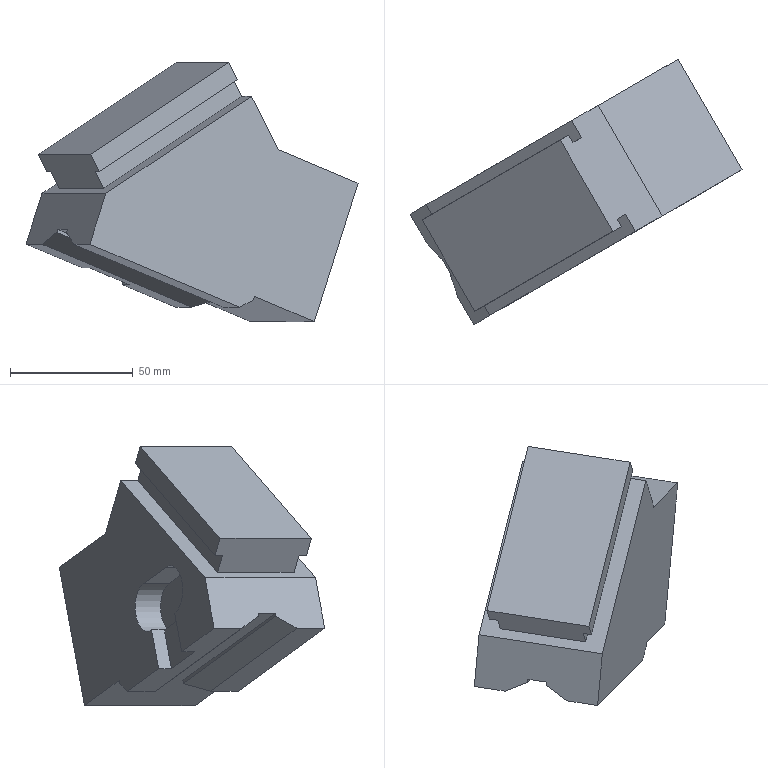Part | NX | features solid 2 | 1 solid | 34 faces | box 135.215 x 108.089 x 105.569 mm | volume 369145 mm3 | plane 32 | cylinder 2 | commonest cylinder face diameters 20 x2
STEP:
#1=CARTESIAN_POINT('',(-359.045,-36.399,34.518));
#2=VERTEX_POINT('',#1);
#3=CARTESIAN_POINT('',(-348.045,-55.451,34.518));
#4=VERTEX_POINT('',#3);
#5=CARTESIAN_POINT('',(-348.045,-55.451,34.518));
#6=DIRECTION('',(0.5,-0.866,0.));
#7=VECTOR('',#6,1000.);
#8=LINE('',#5,#7);
#9=EDGE_CURVE('',#2,#4,#8,.T.);
#10=ORIENTED_EDGE('',*,*,#9,.T.);
#11=CARTESIAN_POINT('',(-348.489,-55.708,33.109));
#12=VERTEX_POINT('',#11);
#13=CARTESIAN_POINT('',(-330.273,-45.191,90.9));
#14=DIRECTION('',(-0.2962,-0.171,-0.9397));
#15=VECTOR('',#14,1000.);
#16=LINE('',#13,#15);
#17=EDGE_CURVE('',#4,#12,#16,.T.);
#18=ORIENTED_EDGE('',*,*,#17,.T.);
#19=CARTESIAN_POINT('',(-359.324,-36.941,33.109));
#20=VERTEX_POINT('',#19);
#21=CARTESIAN_POINT('',(-354.994,-44.441,33.109));
#22=DIRECTION('',(-0.5,0.866,0.));
#23=VECTOR('',#22,1000.);
#24=LINE('',#21,#23);
#25=EDGE_CURVE('',#12,#20,#24,.T.);
#26=ORIENTED_EDGE('',*,*,#25,.T.);
#27=CARTESIAN_POINT('',(-359.432,-36.623,33.288));
#28=VERTEX_POINT('',#27);
#29=CARTESIAN_POINT('',(-362.738,-26.929,38.739));
#30=DIRECTION('',(-0.2849,0.8355,0.4698));
#31=VECTOR('',#30,1000.);
#32=LINE('',#29,#31);
#33=EDGE_CURVE('',#20,#28,#32,.T.);
#34=ORIENTED_EDGE('',*,*,#33,.T.);
#35=CARTESIAN_POINT('',(-341.273,-26.138,90.9));
#36=DIRECTION('',(0.2962,0.171,0.9397));
#37=VECTOR('',#36,1000.);
#38=LINE('',#35,#37);
#39=EDGE_CURVE('',#28,#2,#38,.T.);
#40=ORIENTED_EDGE('',*,*,#39,.T.);
#41=EDGE_LOOP('',(#10,#18,#26,#34,#40));
#42=FACE_BOUND('',#41,.T.);
#43=CARTESIAN_POINT('',(-330.273,-45.191,90.9));
#44=DIRECTION('',(0.8138,0.4698,-0.342));
#45=DIRECTION('',(-0.2962,-0.171,-0.9397));
#46=AXIS2_PLACEMENT_3D('',#43,#44,#45);
#47=PLANE('',#46);
#48=ADVANCED_FACE('',(#42),#47,.T.);
#49=CARTESIAN_POINT('',(-427.486,-50.51,78.471));
#50=VERTEX_POINT('',#49);
#51=CARTESIAN_POINT('',(-409.486,-81.687,78.471));
#52=VERTEX_POINT('',#51);
#53=CARTESIAN_POINT('',(-427.486,-50.51,78.471));
#54=DIRECTION('',(0.5,-0.866,0.));
#55=VECTOR('',#54,1000.);
#56=LINE('',#53,#55);
#57=EDGE_CURVE('',#50,#52,#56,.T.);
#58=ORIENTED_EDGE('',*,*,#57,.F.);
#59=CARTESIAN_POINT('',(-371.236,-18.034,115.971));
#60=VERTEX_POINT('',#59);
#61=CARTESIAN_POINT('',(-427.486,-50.51,78.471));
#62=DIRECTION('',(0.75,0.433,0.5));
#63=VECTOR('',#62,1000.);
#64=LINE('',#61,#63);
#65=EDGE_CURVE('',#50,#60,#64,.T.);
#66=ORIENTED_EDGE('',*,*,#65,.T.);
#67=CARTESIAN_POINT('',(-375.236,-11.106,115.971));
#68=VERTEX_POINT('',#67);
#69=CARTESIAN_POINT('',(-349.236,-56.139,115.971));
#70=DIRECTION('',(-0.5,0.866,0.));
#71=VECTOR('',#70,1000.);
#72=LINE('',#69,#71);
#73=EDGE_CURVE('',#60,#68,#72,.T.);
#74=ORIENTED_EDGE('',*,*,#73,.T.);
#75=CARTESIAN_POINT('',(-434.566,-45.36,76.417));
#76=VERTEX_POINT('',#75);
#77=CARTESIAN_POINT('',(-434.566,-45.36,76.417));
#78=DIRECTION('',(0.75,0.433,0.5));
#79=VECTOR('',#78,1000.);
#80=LINE('',#77,#79);
#81=EDGE_CURVE('',#76,#68,#80,.T.);
#82=ORIENTED_EDGE('',*,*,#81,.F.);
#83=CARTESIAN_POINT('',(-408.566,-90.394,76.417));
#84=VERTEX_POINT('',#83);
#85=CARTESIAN_POINT('',(-408.566,-90.394,76.417));
#86=DIRECTION('',(-0.5,0.866,0.));
#87=VECTOR('',#86,1000.);
#88=LINE('',#85,#87);
#89=EDGE_CURVE('',#84,#76,#88,.T.);
#90=ORIENTED_EDGE('',*,*,#89,.F.);
#91=CARTESIAN_POINT('',(-349.236,-56.139,115.971));
#92=VERTEX_POINT('',#91);
#93=CARTESIAN_POINT('',(-408.566,-90.394,76.417));
#94=DIRECTION('',(0.75,0.433,0.5));
#95=VECTOR('',#94,1000.);
#96=LINE('',#93,#95);
#97=EDGE_CURVE('',#84,#92,#96,.T.);
#98=ORIENTED_EDGE('',*,*,#97,.T.);
#99=CARTESIAN_POINT('',(-353.236,-49.211,115.971));
#100=VERTEX_POINT('',#99);
#101=CARTESIAN_POINT('',(-349.236,-56.139,115.971));
#102=DIRECTION('',(-0.5,0.866,0.));
#103=VECTOR('',#102,1000.);
#104=LINE('',#101,#103);
#105=EDGE_CURVE('',#92,#100,#104,.T.);
#106=ORIENTED_EDGE('',*,*,#105,.T.);
#107=CARTESIAN_POINT('',(-409.486,-81.687,78.471));
#108=DIRECTION('',(0.75,0.433,0.5));
#109=VECTOR('',#108,1000.);
#110=LINE('',#107,#109);
#111=EDGE_CURVE('',#52,#100,#110,.T.);
#112=ORIENTED_EDGE('',*,*,#111,.F.);
#113=EDGE_LOOP('',(#58,#66,#74,#82,#90,#98,#106,#112));
#114=FACE_BOUND('',#113,.T.);
#115=CARTESIAN_POINT('',(-408.566,-90.394,76.417));
#116=DIRECTION('',(-0.433,-0.25,0.866));
#117=DIRECTION('',(0.75,0.433,0.5));
#118=AXIS2_PLACEMENT_3D('',#115,#116,#117);
#119=PLANE('',#118);
#120=ADVANCED_FACE('',(#114),#119,.T.);
#121=CARTESIAN_POINT('',(-360.544,-47.646,30.121));
#122=VERTEX_POINT('',#121);
#123=CARTESIAN_POINT('',(-421.579,-82.884,55.772));
#124=VERTEX_POINT('',#123);
#125=CARTESIAN_POINT('',(-421.579,-82.884,55.772));
#126=DIRECTION('',(-0.8138,-0.4698,0.342));
#127=VECTOR('',#126,1000.);
#128=LINE('',#125,#127);
#129=EDGE_CURVE('',#122,#124,#128,.T.);
#130=ORIENTED_EDGE('',*,*,#129,.F.);
#131=CARTESIAN_POINT('',(-354.039,-58.912,30.121));
#132=VERTEX_POINT('',#131);
#133=CARTESIAN_POINT('',(-354.039,-58.912,30.121));
#134=DIRECTION('',(0.5,-0.866,0.));
#135=VECTOR('',#134,1000.);
#136=LINE('',#133,#135);
#137=EDGE_CURVE('',#122,#132,#136,.T.);
#138=ORIENTED_EDGE('',*,*,#137,.T.);
#139=CARTESIAN_POINT('',(-415.074,-94.151,55.772));
#140=VERTEX_POINT('',#139);
#141=CARTESIAN_POINT('',(-415.074,-94.151,55.772));
#142=DIRECTION('',(0.8138,0.4698,-0.342));
#143=VECTOR('',#142,1000.);
#144=LINE('',#141,#143);
#145=EDGE_CURVE('',#140,#132,#144,.T.);
#146=ORIENTED_EDGE('',*,*,#145,.F.);
#147=CARTESIAN_POINT('',(-415.074,-94.151,55.772));
#148=DIRECTION('',(-0.5,0.866,0.));
#149=VECTOR('',#148,1000.);
#150=LINE('',#147,#149);
#151=EDGE_CURVE('',#140,#124,#150,.T.);
#152=ORIENTED_EDGE('',*,*,#151,.T.);
#153=EDGE_LOOP('',(#130,#138,#146,#152));
#154=FACE_BOUND('',#153,.T.);
#155=CARTESIAN_POINT('',(-415.074,-94.151,55.772));
#156=DIRECTION('',(0.2962,0.171,0.9397));
#157=DIRECTION('',(0.8138,0.4698,-0.342));
#158=AXIS2_PLACEMENT_3D('',#155,#156,#157);
#159=PLANE('',#158);
#160=ADVANCED_FACE('',(#154),#159,.F.);
#161=CARTESIAN_POINT('',(-424.536,-74.21,60.65));
#162=VERTEX_POINT('',#161);
#163=CARTESIAN_POINT('',(-424.536,-74.21,60.65));
#164=DIRECTION('',(0.2849,-0.8355,-0.4698));
#165=VECTOR('',#164,1000.);
#166=LINE('',#163,#165);
#167=EDGE_CURVE('',#162,#124,#166,.T.);
#168=ORIENTED_EDGE('',*,*,#167,.T.);
#169=ORIENTED_EDGE('',*,*,#151,.F.);
#170=CARTESIAN_POINT('',(-408.566,-90.394,76.417));
#171=DIRECTION('',(-0.2962,-0.171,-0.9397));
#172=VECTOR('',#171,1000.);
#173=LINE('',#170,#172);
#174=EDGE_CURVE('',#84,#140,#173,.T.);
#175=ORIENTED_EDGE('',*,*,#174,.F.);
#176=ORIENTED_EDGE('',*,*,#89,.T.);
#177=CARTESIAN_POINT('',(-441.074,-49.117,55.772));
#178=VERTEX_POINT('',#177);
#179=CARTESIAN_POINT('',(-434.566,-45.36,76.417));
#180=DIRECTION('',(-0.2962,-0.171,-0.9397));
#181=VECTOR('',#180,1000.);
#182=LINE('',#179,#181);
#183=EDGE_CURVE('',#76,#178,#182,.T.);
#184=ORIENTED_EDGE('',*,*,#183,.T.);
#185=CARTESIAN_POINT('',(-434.569,-60.384,55.772));
#186=VERTEX_POINT('',#185);
#187=CARTESIAN_POINT('',(-415.074,-94.151,55.772));
#188=DIRECTION('',(-0.5,0.866,0.));
#189=VECTOR('',#188,1000.);
#190=LINE('',#187,#189);
#191=EDGE_CURVE('',#186,#178,#190,.T.);
#192=ORIENTED_EDGE('',*,*,#191,.F.);
#193=CARTESIAN_POINT('',(-428.536,-67.282,60.65));
#194=VERTEX_POINT('',#193);
#195=CARTESIAN_POINT('',(-434.569,-60.384,55.772));
#196=DIRECTION('',(-0.5811,0.6645,-0.4698));
#197=VECTOR('',#196,1000.);
#198=LINE('',#195,#197);
#199=EDGE_CURVE('',#194,#186,#198,.T.);
#200=ORIENTED_EDGE('',*,*,#199,.F.);
#201=CARTESIAN_POINT('',(-428.148,-67.058,61.88));
#202=VERTEX_POINT('',#201);
#203=CARTESIAN_POINT('',(-428.536,-67.282,60.65));
#204=DIRECTION('',(0.2962,0.171,0.9397));
#205=VECTOR('',#204,1000.);
#206=LINE('',#203,#205);
#207=EDGE_CURVE('',#194,#202,#206,.T.);
#208=ORIENTED_EDGE('',*,*,#207,.T.);
#209=CARTESIAN_POINT('',(-424.148,-73.987,61.88));
#210=VERTEX_POINT('',#209);
#211=CARTESIAN_POINT('',(-424.148,-73.987,61.88));
#212=DIRECTION('',(-0.5,0.866,0.));
#213=VECTOR('',#212,1000.);
#214=LINE('',#211,#213);
#215=EDGE_CURVE('',#210,#202,#214,.T.);
#216=ORIENTED_EDGE('',*,*,#215,.F.);
#217=CARTESIAN_POINT('',(-424.148,-73.987,61.88));
#218=DIRECTION('',(-0.2962,-0.171,-0.9397));
#219=VECTOR('',#218,1000.);
#220=LINE('',#217,#219);
#221=EDGE_CURVE('',#210,#162,#220,.T.);
#222=ORIENTED_EDGE('',*,*,#221,.T.);
#223=EDGE_LOOP('',(#168,#169,#175,#176,#184,#192,#200,#208,#216,#222));
#224=FACE_BOUND('',#223,.T.);
#225=CARTESIAN_POINT('',(-408.566,-90.394,76.417));
#226=DIRECTION('',(0.8138,0.4698,-0.342));
#227=DIRECTION('',(-0.2962,-0.171,-0.9397));
#228=AXIS2_PLACEMENT_3D('',#225,#226,#227);
#229=PLANE('',#228);
#230=ADVANCED_FACE('',(#224),#229,.F.);
#231=CARTESIAN_POINT('',(-374.045,-10.418,34.518));
#232=VERTEX_POINT('',#231);
#233=CARTESIAN_POINT('',(-363.045,-29.471,34.518));
#234=VERTEX_POINT('',#233);
#235=CARTESIAN_POINT('',(-348.045,-55.451,34.518));
#236=DIRECTION('',(0.5,-0.866,0.));
#237=VECTOR('',#236,1000.);
#238=LINE('',#235,#237);
#239=EDGE_CURVE('',#232,#234,#238,.T.);
#240=ORIENTED_EDGE('',*,*,#239,.T.);
#241=CARTESIAN_POINT('',(-363.432,-29.695,33.288));
#242=VERTEX_POINT('',#241);
#243=CARTESIAN_POINT('',(-345.273,-19.21,90.9));
#244=DIRECTION('',(-0.2962,-0.171,-0.9397));
#245=VECTOR('',#244,1000.);
#246=LINE('',#243,#245);
#247=EDGE_CURVE('',#234,#242,#246,.T.);
#248=ORIENTED_EDGE('',*,*,#247,.T.);
#249=CARTESIAN_POINT('',(-363.654,-29.441,33.109));
#250=VERTEX_POINT('',#249);
#251=CARTESIAN_POINT('',(-330.521,-67.329,59.898));
#252=DIRECTION('',(0.5811,-0.6645,0.4698));
#253=VECTOR('',#252,1000.);
#254=LINE('',#251,#253);
#255=EDGE_CURVE('',#250,#242,#254,.T.);
#256=ORIENTED_EDGE('',*,*,#255,.F.);
#257=CARTESIAN_POINT('',(-374.489,-10.675,33.109));
#258=VERTEX_POINT('',#257);
#259=CARTESIAN_POINT('',(-374.489,-10.675,33.109));
#260=DIRECTION('',(-0.5,0.866,0.));
#261=VECTOR('',#260,1000.);
#262=LINE('',#259,#261);
#263=EDGE_CURVE('',#250,#258,#262,.T.);
#264=ORIENTED_EDGE('',*,*,#263,.T.);
#265=CARTESIAN_POINT('',(-356.273,-0.1575,90.9));
#266=DIRECTION('',(-0.2962,-0.171,-0.9397));
#267=VECTOR('',#266,1000.);
#268=LINE('',#265,#267);
#269=EDGE_CURVE('',#232,#258,#268,.T.);
#270=ORIENTED_EDGE('',*,*,#269,.F.);
#271=EDGE_LOOP('',(#240,#248,#256,#264,#270));
#272=FACE_BOUND('',#271,.T.);
#273=CARTESIAN_POINT('',(-330.273,-45.191,90.9));
#274=DIRECTION('',(0.8138,0.4698,-0.342));
#275=DIRECTION('',(-0.2962,-0.171,-0.9397));
#276=AXIS2_PLACEMENT_3D('',#273,#274,#275);
#277=PLANE('',#276);
#278=ADVANCED_FACE('',(#272),#277,.T.);
#279=CARTESIAN_POINT('',(-364.411,-4.856,94.32));
#280=VERTEX_POINT('',#279);
#281=CARTESIAN_POINT('',(-331.859,13.938,80.639));
#282=VERTEX_POINT('',#281);
#283=CARTESIAN_POINT('',(-364.411,-4.856,94.32));
#284=DIRECTION('',(0.8138,0.4698,-0.342));
#285=VECTOR('',#284,1000.);
#286=LINE('',#283,#285);
#287=EDGE_CURVE('',#280,#282,#286,.T.);
#288=ORIENTED_EDGE('',*,*,#287,.T.);
#289=CARTESIAN_POINT('',(-349.631,3.677,24.258));
#290=VERTEX_POINT('',#289);
#291=CARTESIAN_POINT('',(-331.859,13.938,80.639));
#292=DIRECTION('',(-0.2962,-0.171,-0.9397));
#293=VECTOR('',#292,1000.);
#294=LINE('',#291,#293);
#295=EDGE_CURVE('',#282,#290,#294,.T.);
#296=ORIENTED_EDGE('',*,*,#295,.T.);
#297=CARTESIAN_POINT('',(-341.493,8.376,20.838));
#298=DIRECTION('',(0.8138,0.4698,-0.342));
#299=VECTOR('',#298,1000.);
#300=LINE('',#297,#299);
#301=EDGE_CURVE('',#290,#232,#300,.F.);
#302=ORIENTED_EDGE('',*,*,#301,.T.);
#303=ORIENTED_EDGE('',*,*,#269,.T.);
#304=CARTESIAN_POINT('',(-380.039,-13.879,30.121));
#305=VERTEX_POINT('',#304);
#306=CARTESIAN_POINT('',(-374.489,-10.675,33.109));
#307=DIRECTION('',(-0.7849,-0.4532,-0.4226));
#308=VECTOR('',#307,1000.);
#309=LINE('',#306,#308);
#310=EDGE_CURVE('',#258,#305,#309,.T.);
#311=ORIENTED_EDGE('',*,*,#310,.T.);
#312=CARTESIAN_POINT('',(-401.933,-26.52,39.322));
#313=VERTEX_POINT('',#312);
#314=CARTESIAN_POINT('',(-441.074,-49.117,55.772));
#315=DIRECTION('',(0.8138,0.4698,-0.342));
#316=VECTOR('',#315,1000.);
#317=LINE('',#314,#316);
#318=EDGE_CURVE('',#313,#305,#317,.T.);
#319=ORIENTED_EDGE('',*,*,#318,.F.);
#320=CARTESIAN_POINT('',(-396.973,-23.656,55.059));
#321=VERTEX_POINT('',#320);
#322=CARTESIAN_POINT('',(-391.049,-20.236,73.853));
#323=DIRECTION('',(-0.2962,-0.171,-0.9397));
#324=VECTOR('',#323,1000.);
#325=LINE('',#322,#324);
#326=EDGE_CURVE('',#321,#313,#325,.T.);
#327=ORIENTED_EDGE('',*,*,#326,.F.);
#328=CARTESIAN_POINT('',(-391.049,-20.236,73.853));
#329=VERTEX_POINT('',#328);
#330=CARTESIAN_POINT('',(-394.011,-21.946,64.456));
#331=DIRECTION('',(0.5,-0.866,0.));
#332=DIRECTION('',(0.866,0.5,0.));
#333=AXIS2_PLACEMENT_3D('',#330,#331,#332);
#334=CIRCLE('',#333,10.);
#335=EDGE_CURVE('',#321,#329,#334,.T.);
#336=ORIENTED_EDGE('',*,*,#335,.T.);
#337=CARTESIAN_POINT('',(-407.325,-29.633,80.694));
#338=VERTEX_POINT('',#337);
#339=CARTESIAN_POINT('',(-391.049,-20.236,73.853));
#340=DIRECTION('',(-0.8138,-0.4698,0.342));
#341=VECTOR('',#340,1000.);
#342=LINE('',#339,#341);
#343=EDGE_CURVE('',#329,#338,#342,.T.);
#344=ORIENTED_EDGE('',*,*,#343,.T.);
#345=CARTESIAN_POINT('',(-413.249,-33.053,61.9));
#346=VERTEX_POINT('',#345);
#347=CARTESIAN_POINT('',(-410.287,-31.343,71.297));
#348=DIRECTION('',(0.5,-0.866,0.));
#349=DIRECTION('',(0.866,0.5,0.));
#350=AXIS2_PLACEMENT_3D('',#347,#348,#349);
#351=CIRCLE('',#350,10.);
#352=EDGE_CURVE('',#338,#346,#351,.T.);
#353=ORIENTED_EDGE('',*,*,#352,.T.);
#354=CARTESIAN_POINT('',(-418.209,-35.917,46.163));
#355=VERTEX_POINT('',#354);
#356=CARTESIAN_POINT('',(-407.325,-29.633,80.694));
#357=DIRECTION('',(-0.2962,-0.171,-0.9397));
#358=VECTOR('',#357,1000.);
#359=LINE('',#356,#358);
#360=EDGE_CURVE('',#346,#355,#359,.T.);
#361=ORIENTED_EDGE('',*,*,#360,.T.);
#362=CARTESIAN_POINT('',(-441.074,-49.117,55.772));
#363=DIRECTION('',(0.8138,0.4698,-0.342));
#364=VECTOR('',#363,1000.);
#365=LINE('',#362,#364);
#366=EDGE_CURVE('',#178,#355,#365,.T.);
#367=ORIENTED_EDGE('',*,*,#366,.F.);
#368=ORIENTED_EDGE('',*,*,#183,.F.);
#369=ORIENTED_EDGE('',*,*,#81,.T.);
#370=CARTESIAN_POINT('',(-375.236,-11.106,115.971));
#371=DIRECTION('',(0.433,0.25,-0.866));
#372=VECTOR('',#371,1000.);
#373=LINE('',#370,#372);
#374=EDGE_CURVE('',#68,#280,#373,.T.);
#375=ORIENTED_EDGE('',*,*,#374,.T.);
#376=EDGE_LOOP('',(#288,#296,#302,#303,#311,#319,#327,#336,#344,#353,#361,#367,#368,#369,#375));
#377=FACE_BOUND('',#376,.T.);
#378=CARTESIAN_POINT('',(-441.074,-49.117,55.772));
#379=DIRECTION('',(0.5,-0.866,0.));
#380=DIRECTION('',(0.,0.,-1.));
#381=AXIS2_PLACEMENT_3D('',#378,#379,#380);
#382=PLANE('',#381);
#383=ADVANCED_FACE('',(#377),#382,.F.);
#384=ORIENTED_EDGE('',*,*,#318,.T.);
#385=CARTESIAN_POINT('',(-373.534,-25.146,30.121));
#386=VERTEX_POINT('',#385);
#387=CARTESIAN_POINT('',(-373.534,-25.146,30.121));
#388=DIRECTION('',(0.5,-0.866,0.));
#389=VECTOR('',#388,1000.);
#390=LINE('',#387,#389);
#391=EDGE_CURVE('',#305,#386,#390,.T.);
#392=ORIENTED_EDGE('',*,*,#391,.T.);
#393=CARTESIAN_POINT('',(-434.569,-60.384,55.772));
#394=DIRECTION('',(-0.8138,-0.4698,0.342));
#395=VECTOR('',#394,1000.);
#396=LINE('',#393,#395);
#397=EDGE_CURVE('',#386,#186,#396,.T.);
#398=ORIENTED_EDGE('',*,*,#397,.T.);
#399=ORIENTED_EDGE('',*,*,#191,.T.);
#400=ORIENTED_EDGE('',*,*,#366,.T.);
#401=CARTESIAN_POINT('',(-415.209,-41.113,46.163));
#402=VERTEX_POINT('',#401);
#403=CARTESIAN_POINT('',(-392.209,-80.95,46.163));
#404=DIRECTION('',(-0.5,0.866,0.));
#405=VECTOR('',#404,1000.);
#406=LINE('',#403,#405);
#407=EDGE_CURVE('',#402,#355,#406,.T.);
#408=ORIENTED_EDGE('',*,*,#407,.F.);
#409=CARTESIAN_POINT('',(-398.933,-31.716,39.322));
#410=VERTEX_POINT('',#409);
#411=CARTESIAN_POINT('',(-438.074,-54.314,55.772));
#412=DIRECTION('',(-0.8138,-0.4698,0.342));
#413=VECTOR('',#412,1000.);
#414=LINE('',#411,#413);
#415=EDGE_CURVE('',#410,#402,#414,.T.);
#416=ORIENTED_EDGE('',*,*,#415,.F.);
#417=CARTESIAN_POINT('',(-375.933,-71.553,39.322));
#418=DIRECTION('',(-0.5,0.866,0.));
#419=VECTOR('',#418,1000.);
#420=LINE('',#417,#419);
#421=EDGE_CURVE('',#410,#313,#420,.T.);
#422=ORIENTED_EDGE('',*,*,#421,.T.);
#423=EDGE_LOOP('',(#384,#392,#398,#399,#400,#408,#416,#422));
#424=FACE_BOUND('',#423,.T.);
#425=CARTESIAN_POINT('',(-415.074,-94.151,55.772));
#426=DIRECTION('',(0.2962,0.171,0.9397));
#427=DIRECTION('',(0.8138,0.4698,-0.342));
#428=AXIS2_PLACEMENT_3D('',#425,#426,#427);
#429=PLANE('',#428);
#430=ADVANCED_FACE('',(#424),#429,.F.);
#431=CARTESIAN_POINT('',(-393.973,-28.852,55.059));
#432=VERTEX_POINT('',#431);
#433=CARTESIAN_POINT('',(-410.249,-38.249,61.9));
#434=VERTEX_POINT('',#433);
#435=CARTESIAN_POINT('',(-393.973,-28.852,55.059));
#436=DIRECTION('',(-0.8138,-0.4698,0.342));
#437=VECTOR('',#436,1000.);
#438=LINE('',#435,#437);
#439=EDGE_CURVE('',#432,#434,#438,.T.);
#440=ORIENTED_EDGE('',*,*,#439,.T.);
#441=CARTESIAN_POINT('',(-407.249,-43.445,61.9));
#442=VERTEX_POINT('',#441);
#443=CARTESIAN_POINT('',(-407.249,-43.445,61.9));
#444=DIRECTION('',(-0.5,0.866,0.));
#445=VECTOR('',#444,1000.);
#446=LINE('',#443,#445);
#447=EDGE_CURVE('',#442,#434,#446,.T.);
#448=ORIENTED_EDGE('',*,*,#447,.F.);
#449=CARTESIAN_POINT('',(-390.973,-34.048,55.059));
#450=VERTEX_POINT('',#449);
#451=CARTESIAN_POINT('',(-390.973,-34.048,55.059));
#452=DIRECTION('',(-0.8138,-0.4698,0.342));
#453=VECTOR('',#452,1000.);
#454=LINE('',#451,#453);
#455=EDGE_CURVE('',#450,#442,#454,.T.);
#456=ORIENTED_EDGE('',*,*,#455,.F.);
#457=CARTESIAN_POINT('',(-390.973,-34.048,55.059));
#458=DIRECTION('',(-0.5,0.866,0.));
#459=VECTOR('',#458,1000.);
#460=LINE('',#457,#459);
#461=EDGE_CURVE('',#450,#432,#460,.T.);
#462=ORIENTED_EDGE('',*,*,#461,.T.);
#463=EDGE_LOOP('',(#440,#448,#456,#462));
#464=FACE_BOUND('',#463,.T.);
#465=CARTESIAN_POINT('',(-390.973,-34.048,55.059));
#466=DIRECTION('',(-0.2962,-0.171,-0.9397));
#467=DIRECTION('',(-0.8138,-0.4698,0.342));
#468=AXIS2_PLACEMENT_3D('',#465,#466,#467);
#469=PLANE('',#468);
#470=ADVANCED_FACE('',(#464),#469,.F.);
#471=ORIENTED_EDGE('',*,*,#287,.F.);
#472=CARTESIAN_POINT('',(-338.411,-49.889,94.32));
#473=VERTEX_POINT('',#472);
#474=CARTESIAN_POINT('',(-338.411,-49.889,94.32));
#475=DIRECTION('',(-0.5,0.866,0.));
#476=VECTOR('',#475,1000.);
#477=LINE('',#474,#476);
#478=EDGE_CURVE('',#473,#280,#477,.T.);
#479=ORIENTED_EDGE('',*,*,#478,.F.);
#480=CARTESIAN_POINT('',(-305.859,-31.095,80.639));
#481=VERTEX_POINT('',#480);
#482=CARTESIAN_POINT('',(-338.411,-49.889,94.32));
#483=DIRECTION('',(0.8138,0.4698,-0.342));
#484=VECTOR('',#483,1000.);
#485=LINE('',#482,#484);
#486=EDGE_CURVE('',#473,#481,#485,.T.);
#487=ORIENTED_EDGE('',*,*,#486,.T.);
#488=CARTESIAN_POINT('',(-305.859,-31.095,80.639));
#489=DIRECTION('',(-0.5,0.866,0.));
#490=VECTOR('',#489,1000.);
#491=LINE('',#488,#490);
#492=EDGE_CURVE('',#481,#282,#491,.T.);
#493=ORIENTED_EDGE('',*,*,#492,.T.);
#494=EDGE_LOOP('',(#471,#479,#487,#493));
#495=FACE_BOUND('',#494,.T.);
#496=CARTESIAN_POINT('',(-338.411,-49.889,94.32));
#497=DIRECTION('',(0.2962,0.171,0.9397));
#498=DIRECTION('',(0.8138,0.4698,-0.342));
#499=AXIS2_PLACEMENT_3D('',#496,#497,#498);
#500=PLANE('',#499);
#501=ADVANCED_FACE('',(#495),#500,.T.);
#502=ORIENTED_EDGE('',*,*,#374,.F.);
#503=ORIENTED_EDGE('',*,*,#73,.F.);
#504=CARTESIAN_POINT('',(-374.7,-20.034,122.899));
#505=VERTEX_POINT('',#504);
#506=CARTESIAN_POINT('',(-374.7,-20.034,122.899));
#507=DIRECTION('',(0.433,0.25,-0.866));
#508=VECTOR('',#507,1000.);
#509=LINE('',#506,#508);
#510=EDGE_CURVE('',#505,#60,#509,.T.);
#511=ORIENTED_EDGE('',*,*,#510,.F.);
#512=CARTESIAN_POINT('',(-376.45,-17.003,122.899));
#513=VERTEX_POINT('',#512);
#514=CARTESIAN_POINT('',(-376.45,-17.003,122.899));
#515=DIRECTION('',(0.5,-0.866,0.));
#516=VECTOR('',#515,1000.);
#517=LINE('',#514,#516);
#518=EDGE_CURVE('',#513,#505,#517,.T.);
#519=ORIENTED_EDGE('',*,*,#518,.F.);
#520=CARTESIAN_POINT('',(-379.914,-19.003,129.827));
#521=VERTEX_POINT('',#520);
#522=CARTESIAN_POINT('',(-379.914,-19.003,129.827));
#523=DIRECTION('',(0.433,0.25,-0.866));
#524=VECTOR('',#523,1000.);
#525=LINE('',#522,#524);
#526=EDGE_CURVE('',#521,#513,#525,.T.);
#527=ORIENTED_EDGE('',*,*,#526,.F.);
#528=CARTESIAN_POINT('',(-358.414,-56.242,129.827));
#529=VERTEX_POINT('',#528);
#530=CARTESIAN_POINT('',(-379.914,-19.003,129.827));
#531=DIRECTION('',(0.5,-0.866,0.));
#532=VECTOR('',#531,1000.);
#533=LINE('',#530,#532);
#534=EDGE_CURVE('',#521,#529,#533,.T.);
#535=ORIENTED_EDGE('',*,*,#534,.T.);
#536=CARTESIAN_POINT('',(-354.95,-54.242,122.899));
#537=VERTEX_POINT('',#536);
#538=CARTESIAN_POINT('',(-358.414,-56.242,129.827));
#539=DIRECTION('',(0.433,0.25,-0.866));
#540=VECTOR('',#539,1000.);
#541=LINE('',#538,#540);
#542=EDGE_CURVE('',#529,#537,#541,.T.);
#543=ORIENTED_EDGE('',*,*,#542,.T.);
#544=CARTESIAN_POINT('',(-356.7,-51.211,122.899));
#545=VERTEX_POINT('',#544);
#546=CARTESIAN_POINT('',(-376.45,-17.003,122.899));
#547=DIRECTION('',(0.5,-0.866,0.));
#548=VECTOR('',#547,1000.);
#549=LINE('',#546,#548);
#550=EDGE_CURVE('',#545,#537,#549,.T.);
#551=ORIENTED_EDGE('',*,*,#550,.F.);
#552=CARTESIAN_POINT('',(-356.7,-51.211,122.899));
#553=DIRECTION('',(0.433,0.25,-0.866));
#554=VECTOR('',#553,1000.);
#555=LINE('',#552,#554);
#556=EDGE_CURVE('',#545,#100,#555,.T.);
#557=ORIENTED_EDGE('',*,*,#556,.T.);
#558=ORIENTED_EDGE('',*,*,#105,.F.);
#559=CARTESIAN_POINT('',(-349.236,-56.139,115.971));
#560=DIRECTION('',(0.433,0.25,-0.866));
#561=VECTOR('',#560,1000.);
#562=LINE('',#559,#561);
#563=EDGE_CURVE('',#92,#473,#562,.T.);
#564=ORIENTED_EDGE('',*,*,#563,.T.);
#565=ORIENTED_EDGE('',*,*,#478,.T.);
#566=EDGE_LOOP('',(#502,#503,#511,#519,#527,#535,#543,#551,#557,#558,#564,#565));
#567=FACE_BOUND('',#566,.T.);
#568=CARTESIAN_POINT('',(-349.236,-56.139,115.971));
#569=DIRECTION('',(0.75,0.433,0.5));
#570=DIRECTION('',(0.433,0.25,-0.866));
#571=AXIS2_PLACEMENT_3D('',#568,#569,#570);
#572=PLANE('',#571);
#573=ADVANCED_FACE('',(#567),#572,.T.);
#574=ORIENTED_EDGE('',*,*,#145,.T.);
#575=CARTESIAN_POINT('',(-395.664,-82.944,7.708));
#576=DIRECTION('',(0.7849,0.4532,0.4226));
#577=VECTOR('',#576,1000.);
#578=LINE('',#575,#577);
#579=EDGE_CURVE('',#132,#12,#578,.T.);
#580=ORIENTED_EDGE('',*,*,#579,.T.);
#581=ORIENTED_EDGE('',*,*,#17,.F.);
#582=CARTESIAN_POINT('',(-323.631,-41.356,24.258));
#583=VERTEX_POINT('',#582);
#584=CARTESIAN_POINT('',(-315.493,-36.658,20.838));
#585=DIRECTION('',(0.8138,0.4698,-0.342));
#586=VECTOR('',#585,1000.);
#587=LINE('',#584,#586);
#588=EDGE_CURVE('',#583,#4,#587,.F.);
#589=ORIENTED_EDGE('',*,*,#588,.F.);
#590=CARTESIAN_POINT('',(-305.859,-31.095,80.639));
#591=DIRECTION('',(-0.2962,-0.171,-0.9397));
#592=VECTOR('',#591,1000.);
#593=LINE('',#590,#592);
#594=EDGE_CURVE('',#481,#583,#593,.T.);
#595=ORIENTED_EDGE('',*,*,#594,.F.);
#596=ORIENTED_EDGE('',*,*,#486,.F.);
#597=ORIENTED_EDGE('',*,*,#563,.F.);
#598=ORIENTED_EDGE('',*,*,#97,.F.);
#599=ORIENTED_EDGE('',*,*,#174,.T.);
#600=EDGE_LOOP('',(#574,#580,#581,#589,#595,#596,#597,#598,#599));
#601=FACE_BOUND('',#600,.T.);
#602=CARTESIAN_POINT('',(-415.074,-94.151,55.772));
#603=DIRECTION('',(0.5,-0.866,0.));
#604=DIRECTION('',(0.,0.,-1.));
#605=AXIS2_PLACEMENT_3D('',#602,#603,#604);
#606=PLANE('',#605);
#607=ADVANCED_FACE('',(#601),#606,.T.);
#608=ORIENTED_EDGE('',*,*,#343,.F.);
#609=CARTESIAN_POINT('',(-385.049,-30.628,73.853));
#610=VERTEX_POINT('',#609);
#611=CARTESIAN_POINT('',(-385.049,-30.628,73.853));
#612=DIRECTION('',(-0.5,0.866,0.));
#613=VECTOR('',#612,1000.);
#614=LINE('',#611,#613);
#615=EDGE_CURVE('',#610,#329,#614,.T.);
#616=ORIENTED_EDGE('',*,*,#615,.F.);
#617=CARTESIAN_POINT('',(-401.325,-40.025,80.694));
#618=VERTEX_POINT('',#617);
#619=CARTESIAN_POINT('',(-385.049,-30.628,73.853));
#620=DIRECTION('',(-0.8138,-0.4698,0.342));
#621=VECTOR('',#620,1000.);
#622=LINE('',#619,#621);
#623=EDGE_CURVE('',#610,#618,#622,.T.);
#624=ORIENTED_EDGE('',*,*,#623,.T.);
#625=CARTESIAN_POINT('',(-401.325,-40.025,80.694));
#626=DIRECTION('',(-0.5,0.866,0.));
#627=VECTOR('',#626,1000.);
#628=LINE('',#625,#627);
#629=EDGE_CURVE('',#618,#338,#628,.T.);
#630=ORIENTED_EDGE('',*,*,#629,.T.);
#631=EDGE_LOOP('',(#608,#616,#624,#630));
#632=FACE_BOUND('',#631,.T.);
#633=CARTESIAN_POINT('',(-385.049,-30.628,73.853));
#634=DIRECTION('',(-0.2962,-0.171,-0.9397));
#635=DIRECTION('',(-0.8138,-0.4698,0.342));
#636=AXIS2_PLACEMENT_3D('',#633,#634,#635);
#637=PLANE('',#636);
#638=ADVANCED_FACE('',(#632),#637,.T.);
#639=ORIENTED_EDGE('',*,*,#352,.F.);
#640=ORIENTED_EDGE('',*,*,#629,.F.);
#641=CARTESIAN_POINT('',(-404.287,-41.735,71.297));
#642=DIRECTION('',(0.5,-0.866,0.));
#643=DIRECTION('',(0.866,0.5,0.));
#644=AXIS2_PLACEMENT_3D('',#641,#642,#643);
#645=CIRCLE('',#644,10.);
#646=EDGE_CURVE('',#618,#442,#645,.T.);
#647=ORIENTED_EDGE('',*,*,#646,.T.);
#648=ORIENTED_EDGE('',*,*,#447,.T.);
#649=CARTESIAN_POINT('',(-407.249,-43.445,61.9));
#650=DIRECTION('',(0.5,-0.866,0.));
#651=VECTOR('',#650,1000.);
#652=LINE('',#649,#651);
#653=EDGE_CURVE('',#346,#434,#652,.T.);
#654=ORIENTED_EDGE('',*,*,#653,.F.);
#655=EDGE_LOOP('',(#639,#640,#647,#648,#654));
#656=FACE_BOUND('',#655,.T.);
#657=CARTESIAN_POINT('',(-404.287,-41.735,71.297));
#658=DIRECTION('',(-0.5,0.866,0.));
#659=DIRECTION('',(0.,0.,1.));
#660=AXIS2_PLACEMENT_3D('',#657,#658,#659);
#661=CYLINDRICAL_SURFACE('',#660,10.);
#662=ADVANCED_FACE('',(#656),#661,.F.);
#663=ORIENTED_EDGE('',*,*,#335,.F.);
#664=CARTESIAN_POINT('',(-390.973,-34.048,55.059));
#665=DIRECTION('',(-0.5,0.866,0.));
#666=VECTOR('',#665,1000.);
#667=LINE('',#664,#666);
#668=EDGE_CURVE('',#432,#321,#667,.T.);
#669=ORIENTED_EDGE('',*,*,#668,.F.);
#670=ORIENTED_EDGE('',*,*,#461,.F.);
#671=CARTESIAN_POINT('',(-388.011,-32.338,64.456));
#672=DIRECTION('',(0.5,-0.866,0.));
#673=DIRECTION('',(0.866,0.5,0.));
#674=AXIS2_PLACEMENT_3D('',#671,#672,#673);
#675=CIRCLE('',#674,10.);
#676=EDGE_CURVE('',#450,#610,#675,.T.);
#677=ORIENTED_EDGE('',*,*,#676,.T.);
#678=ORIENTED_EDGE('',*,*,#615,.T.);
#679=EDGE_LOOP('',(#663,#669,#670,#677,#678));
#680=FACE_BOUND('',#679,.T.);
#681=CARTESIAN_POINT('',(-388.011,-32.338,64.456));
#682=DIRECTION('',(-0.5,0.866,0.));
#683=DIRECTION('',(0.,0.,1.));
#684=AXIS2_PLACEMENT_3D('',#681,#682,#683);
#685=CYLINDRICAL_SURFACE('',#684,10.);
#686=ADVANCED_FACE('',(#680),#685,.F.);
#687=ORIENTED_EDGE('',*,*,#676,.F.);
#688=ORIENTED_EDGE('',*,*,#455,.T.);
#689=ORIENTED_EDGE('',*,*,#646,.F.);
#690=ORIENTED_EDGE('',*,*,#623,.F.);
#691=EDGE_LOOP('',(#687,#688,#689,#690));
#692=FACE_BOUND('',#691,.T.);
#693=CARTESIAN_POINT('',(-404.287,-41.735,71.297));
#694=DIRECTION('',(0.5,-0.866,0.));
#695=DIRECTION('',(0.,0.,-1.));
#696=AXIS2_PLACEMENT_3D('',#693,#694,#695);
#697=PLANE('',#696);
#698=ADVANCED_FACE('',(#692),#697,.F.);
#699=ORIENTED_EDGE('',*,*,#415,.T.);
#700=CARTESIAN_POINT('',(-417.062,-42.182,40.287));
#701=DIRECTION('',(0.2962,0.171,0.9397));
#702=VECTOR('',#701,1000.);
#703=LINE('',#700,#702);
#704=EDGE_CURVE('',#402,#434,#703,.T.);
#705=ORIENTED_EDGE('',*,*,#704,.T.);
#706=ORIENTED_EDGE('',*,*,#439,.F.);
#707=CARTESIAN_POINT('',(-400.786,-32.785,33.446));
#708=DIRECTION('',(0.2962,0.171,0.9397));
#709=VECTOR('',#708,1000.);
#710=LINE('',#707,#709);
#711=EDGE_CURVE('',#410,#432,#710,.T.);
#712=ORIENTED_EDGE('',*,*,#711,.F.);
#713=EDGE_LOOP('',(#699,#705,#706,#712));
#714=FACE_BOUND('',#713,.T.);
#715=CARTESIAN_POINT('',(-417.062,-42.182,40.287));
#716=DIRECTION('',(-0.5,0.866,0.));
#717=DIRECTION('',(0.,0.,1.));
#718=AXIS2_PLACEMENT_3D('',#715,#716,#717);
#719=PLANE('',#718);
#720=ADVANCED_FACE('',(#714),#719,.T.);
#721=ORIENTED_EDGE('',*,*,#407,.T.);
#722=ORIENTED_EDGE('',*,*,#360,.F.);
#723=ORIENTED_EDGE('',*,*,#653,.T.);
#724=ORIENTED_EDGE('',*,*,#704,.F.);
#725=EDGE_LOOP('',(#721,#722,#723,#724));
#726=FACE_BOUND('',#725,.T.);
#727=CARTESIAN_POINT('',(-404.325,-34.829,80.694));
#728=DIRECTION('',(0.8138,0.4698,-0.342));
#729=DIRECTION('',(0.2962,0.171,0.9397));
#730=AXIS2_PLACEMENT_3D('',#727,#728,#729);
#731=PLANE('',#730);
#732=ADVANCED_FACE('',(#726),#731,.T.);
#733=ORIENTED_EDGE('',*,*,#711,.T.);
#734=ORIENTED_EDGE('',*,*,#668,.T.);
#735=ORIENTED_EDGE('',*,*,#326,.T.);
#736=ORIENTED_EDGE('',*,*,#421,.F.);
#737=EDGE_LOOP('',(#733,#734,#735,#736));
#738=FACE_BOUND('',#737,.T.);
#739=CARTESIAN_POINT('',(-388.049,-25.432,73.853));
#740=DIRECTION('',(0.8138,0.4698,-0.342));
#741=DIRECTION('',(0.2962,0.171,0.9397));
#742=AXIS2_PLACEMENT_3D('',#739,#740,#741);
#743=PLANE('',#742);
#744=ADVANCED_FACE('',(#738),#743,.F.);
#745=ORIENTED_EDGE('',*,*,#33,.F.);
#746=CARTESIAN_POINT('',(-358.799,-32.333,34.395));
#747=DIRECTION('',(-0.1091,-0.9574,-0.2673));
#748=VECTOR('',#747,1000.);
#749=LINE('',#746,#748);
#750=EDGE_CURVE('',#20,#122,#749,.T.);
#751=ORIENTED_EDGE('',*,*,#750,.T.);
#752=ORIENTED_EDGE('',*,*,#129,.T.);
#753=ORIENTED_EDGE('',*,*,#167,.F.);
#754=CARTESIAN_POINT('',(-351.295,-31.924,29.868));
#755=DIRECTION('',(-0.8138,-0.4698,0.342));
#756=VECTOR('',#755,1000.);
#757=LINE('',#754,#756);
#758=EDGE_CURVE('',#28,#162,#757,.T.);
#759=ORIENTED_EDGE('',*,*,#758,.F.);
#760=EDGE_LOOP('',(#745,#751,#752,#753,#759));
#761=FACE_BOUND('',#760,.T.);
#762=CARTESIAN_POINT('',(-351.295,-31.924,29.868));
#763=DIRECTION('',(-0.5065,0.2849,-0.8138));
#764=DIRECTION('',(-0.426,0.7379,0.5235));
#765=AXIS2_PLACEMENT_3D('',#762,#763,#764);
#766=PLANE('',#765);
#767=ADVANCED_FACE('',(#761),#766,.T.);
#768=ORIENTED_EDGE('',*,*,#397,.F.);
#769=CARTESIAN_POINT('',(-342.893,-38.468,39.388));
#770=DIRECTION('',(0.8837,-0.3842,0.2673));
#771=VECTOR('',#770,1000.);
#772=LINE('',#769,#771);
#773=EDGE_CURVE('',#386,#250,#772,.T.);
#774=ORIENTED_EDGE('',*,*,#773,.T.);
#775=ORIENTED_EDGE('',*,*,#255,.T.);
#776=CARTESIAN_POINT('',(-355.295,-24.996,29.868));
#777=DIRECTION('',(-0.8138,-0.4698,0.342));
#778=VECTOR('',#777,1000.);
#779=LINE('',#776,#778);
#780=EDGE_CURVE('',#242,#194,#779,.T.);
#781=ORIENTED_EDGE('',*,*,#780,.T.);
#782=ORIENTED_EDGE('',*,*,#199,.T.);
#783=EDGE_LOOP('',(#768,#774,#775,#781,#782));
#784=FACE_BOUND('',#783,.T.);
#785=CARTESIAN_POINT('',(-361.327,-18.098,24.99));
#786=DIRECTION('',(0.006515,0.5811,0.8138));
#787=DIRECTION('',(0.426,-0.7379,0.5235));
#788=AXIS2_PLACEMENT_3D('',#785,#786,#787);
#789=PLANE('',#788);
#790=ADVANCED_FACE('',(#784),#789,.F.);
#791=CARTESIAN_POINT('',(-354.907,-24.772,31.098));
#792=DIRECTION('',(-0.8138,-0.4698,0.342));
#793=VECTOR('',#792,1000.);
#794=LINE('',#791,#793);
#795=EDGE_CURVE('',#234,#202,#794,.T.);
#796=ORIENTED_EDGE('',*,*,#795,.F.);
#797=ORIENTED_EDGE('',*,*,#239,.F.);
#798=ORIENTED_EDGE('',*,*,#301,.F.);
#799=CARTESIAN_POINT('',(-323.631,-41.356,24.258));
#800=DIRECTION('',(0.5,-0.866,0.));
#801=VECTOR('',#800,1000.);
#802=LINE('',#799,#801);
#803=EDGE_CURVE('',#583,#290,#802,.F.);
#804=ORIENTED_EDGE('',*,*,#803,.F.);
#805=ORIENTED_EDGE('',*,*,#588,.T.);
#806=ORIENTED_EDGE('',*,*,#9,.F.);
#807=CARTESIAN_POINT('',(-350.907,-31.7,31.098));
#808=DIRECTION('',(-0.8138,-0.4698,0.342));
#809=VECTOR('',#808,1000.);
#810=LINE('',#807,#809);
#811=EDGE_CURVE('',#2,#210,#810,.T.);
#812=ORIENTED_EDGE('',*,*,#811,.T.);
#813=ORIENTED_EDGE('',*,*,#215,.T.);
#814=EDGE_LOOP('',(#796,#797,#798,#804,#805,#806,#812,#813));
#815=FACE_BOUND('',#814,.T.);
#816=CARTESIAN_POINT('',(-350.907,-31.7,31.098));
#817=DIRECTION('',(0.2962,0.171,0.9397));
#818=DIRECTION('',(0.8138,0.4698,-0.342));
#819=AXIS2_PLACEMENT_3D('',#816,#817,#818);
#820=PLANE('',#819);
#821=ADVANCED_FACE('',(#815),#820,.F.);
#822=ORIENTED_EDGE('',*,*,#247,.F.);
#823=ORIENTED_EDGE('',*,*,#795,.T.);
#824=ORIENTED_EDGE('',*,*,#207,.F.);
#825=ORIENTED_EDGE('',*,*,#780,.F.);
#826=EDGE_LOOP('',(#822,#823,#824,#825));
#827=FACE_BOUND('',#826,.T.);
#828=CARTESIAN_POINT('',(-355.295,-24.996,29.868));
#829=DIRECTION('',(0.5,-0.866,0.));
#830=DIRECTION('',(0.,0.,-1.));
#831=AXIS2_PLACEMENT_3D('',#828,#829,#830);
#832=PLANE('',#831);
#833=ADVANCED_FACE('',(#827),#832,.T.);
#834=ORIENTED_EDGE('',*,*,#39,.F.);
#835=ORIENTED_EDGE('',*,*,#758,.T.);
#836=ORIENTED_EDGE('',*,*,#221,.F.);
#837=ORIENTED_EDGE('',*,*,#811,.F.);
#838=EDGE_LOOP('',(#834,#835,#836,#837));
#839=FACE_BOUND('',#838,.T.);
#840=CARTESIAN_POINT('',(-350.907,-31.7,31.098));
#841=DIRECTION('',(-0.5,0.866,0.));
#842=DIRECTION('',(0.,0.,1.));
#843=AXIS2_PLACEMENT_3D('',#840,#841,#842);
#844=PLANE('',#843);
#845=ADVANCED_FACE('',(#839),#844,.T.);
#846=CARTESIAN_POINT('',(-412.95,-83.687,85.399));
#847=VERTEX_POINT('',#846);
#848=CARTESIAN_POINT('',(-412.95,-83.687,85.399));
#849=DIRECTION('',(0.433,0.25,-0.866));
#850=VECTOR('',#849,1000.);
#851=LINE('',#848,#850);
#852=EDGE_CURVE('',#847,#52,#851,.T.);
#853=ORIENTED_EDGE('',*,*,#852,.F.);
#854=CARTESIAN_POINT('',(-411.2,-86.718,85.399));
#855=VERTEX_POINT('',#854);
#856=CARTESIAN_POINT('',(-432.7,-49.479,85.399));
#857=DIRECTION('',(0.5,-0.866,0.));
#858=VECTOR('',#857,1000.);
#859=LINE('',#856,#858);
#860=EDGE_CURVE('',#847,#855,#859,.T.);
#861=ORIENTED_EDGE('',*,*,#860,.T.);
#862=CARTESIAN_POINT('',(-414.664,-88.718,92.327));
#863=VERTEX_POINT('',#862);
#864=CARTESIAN_POINT('',(-414.664,-88.718,92.327));
#865=DIRECTION('',(0.433,0.25,-0.866));
#866=VECTOR('',#865,1000.);
#867=LINE('',#864,#866);
#868=EDGE_CURVE('',#863,#855,#867,.T.);
#869=ORIENTED_EDGE('',*,*,#868,.F.);
#870=CARTESIAN_POINT('',(-436.164,-51.479,92.327));
#871=VERTEX_POINT('',#870);
#872=CARTESIAN_POINT('',(-436.164,-51.479,92.327));
#873=DIRECTION('',(0.5,-0.866,0.));
#874=VECTOR('',#873,1000.);
#875=LINE('',#872,#874);
#876=EDGE_CURVE('',#871,#863,#875,.T.);
#877=ORIENTED_EDGE('',*,*,#876,.F.);
#878=CARTESIAN_POINT('',(-432.7,-49.479,85.399));
#879=VERTEX_POINT('',#878);
#880=CARTESIAN_POINT('',(-436.164,-51.479,92.327));
#881=DIRECTION('',(0.433,0.25,-0.866));
#882=VECTOR('',#881,1000.);
#883=LINE('',#880,#882);
#884=EDGE_CURVE('',#871,#879,#883,.T.);
#885=ORIENTED_EDGE('',*,*,#884,.T.);
#886=CARTESIAN_POINT('',(-430.95,-52.51,85.399));
#887=VERTEX_POINT('',#886);
#888=CARTESIAN_POINT('',(-432.7,-49.479,85.399));
#889=DIRECTION('',(0.5,-0.866,0.));
#890=VECTOR('',#889,1000.);
#891=LINE('',#888,#890);
#892=EDGE_CURVE('',#879,#887,#891,.T.);
#893=ORIENTED_EDGE('',*,*,#892,.T.);
#894=CARTESIAN_POINT('',(-430.95,-52.51,85.399));
#895=DIRECTION('',(0.433,0.25,-0.866));
#896=VECTOR('',#895,1000.);
#897=LINE('',#894,#896);
#898=EDGE_CURVE('',#887,#50,#897,.T.);
#899=ORIENTED_EDGE('',*,*,#898,.T.);
#900=ORIENTED_EDGE('',*,*,#57,.T.);
#901=EDGE_LOOP('',(#853,#861,#869,#877,#885,#893,#899,#900));
#902=FACE_BOUND('',#901,.T.);
#903=CARTESIAN_POINT('',(-430.95,-52.51,85.399));
#904=DIRECTION('',(-0.75,-0.433,-0.5));
#905=DIRECTION('',(-0.433,-0.25,0.866));
#906=AXIS2_PLACEMENT_3D('',#903,#904,#905);
#907=PLANE('',#906);
#908=ADVANCED_FACE('',(#902),#907,.T.);
#909=CARTESIAN_POINT('',(-374.7,-20.034,122.899));
#910=DIRECTION('',(-0.75,-0.433,-0.5));
#911=VECTOR('',#910,1000.);
#912=LINE('',#909,#911);
#913=EDGE_CURVE('',#505,#887,#912,.T.);
#914=ORIENTED_EDGE('',*,*,#913,.F.);
#915=ORIENTED_EDGE('',*,*,#510,.T.);
#916=ORIENTED_EDGE('',*,*,#65,.F.);
#917=ORIENTED_EDGE('',*,*,#898,.F.);
#918=EDGE_LOOP('',(#914,#915,#916,#917));
#919=FACE_BOUND('',#918,.T.);
#920=CARTESIAN_POINT('',(-430.95,-52.51,85.399));
#921=DIRECTION('',(0.5,-0.866,0.));
#922=DIRECTION('',(0.,0.,-1.));
#923=AXIS2_PLACEMENT_3D('',#920,#921,#922);
#924=PLANE('',#923);
#925=ADVANCED_FACE('',(#919),#924,.F.);
#926=CARTESIAN_POINT('',(-356.7,-51.211,122.899));
#927=DIRECTION('',(-0.75,-0.433,-0.5));
#928=VECTOR('',#927,1000.);
#929=LINE('',#926,#928);
#930=EDGE_CURVE('',#545,#847,#929,.T.);
#931=ORIENTED_EDGE('',*,*,#930,.T.);
#932=ORIENTED_EDGE('',*,*,#852,.T.);
#933=ORIENTED_EDGE('',*,*,#111,.T.);
#934=ORIENTED_EDGE('',*,*,#556,.F.);
#935=EDGE_LOOP('',(#931,#932,#933,#934));
#936=FACE_BOUND('',#935,.T.);
#937=CARTESIAN_POINT('',(-412.95,-83.687,85.399));
#938=DIRECTION('',(0.5,-0.866,0.));
#939=DIRECTION('',(0.,0.,-1.));
#940=AXIS2_PLACEMENT_3D('',#937,#938,#939);
#941=PLANE('',#940);
#942=ADVANCED_FACE('',(#936),#941,.T.);
#943=ORIENTED_EDGE('',*,*,#518,.T.);
#944=ORIENTED_EDGE('',*,*,#913,.T.);
#945=ORIENTED_EDGE('',*,*,#892,.F.);
#946=CARTESIAN_POINT('',(-376.45,-17.003,122.899));
#947=DIRECTION('',(-0.75,-0.433,-0.5));
#948=VECTOR('',#947,1000.);
#949=LINE('',#946,#948);
#950=EDGE_CURVE('',#513,#879,#949,.T.);
#951=ORIENTED_EDGE('',*,*,#950,.F.);
#952=EDGE_LOOP('',(#943,#944,#945,#951));
#953=FACE_BOUND('',#952,.T.);
#954=CARTESIAN_POINT('',(-376.45,-17.003,122.899));
#955=DIRECTION('',(-0.433,-0.25,0.866));
#956=DIRECTION('',(0.75,0.433,0.5));
#957=AXIS2_PLACEMENT_3D('',#954,#955,#956);
#958=PLANE('',#957);
#959=ADVANCED_FACE('',(#953),#958,.F.);
#960=ORIENTED_EDGE('',*,*,#930,.F.);
#961=ORIENTED_EDGE('',*,*,#550,.T.);
#962=CARTESIAN_POINT('',(-354.95,-54.242,122.899));
#963=DIRECTION('',(-0.75,-0.433,-0.5));
#964=VECTOR('',#963,1000.);
#965=LINE('',#962,#964);
#966=EDGE_CURVE('',#537,#855,#965,.T.);
#967=ORIENTED_EDGE('',*,*,#966,.T.);
#968=ORIENTED_EDGE('',*,*,#860,.F.);
#969=EDGE_LOOP('',(#960,#961,#967,#968));
#970=FACE_BOUND('',#969,.T.);
#971=CARTESIAN_POINT('',(-376.45,-17.003,122.899));
#972=DIRECTION('',(-0.433,-0.25,0.866));
#973=DIRECTION('',(0.75,0.433,0.5));
#974=AXIS2_PLACEMENT_3D('',#971,#972,#973);
#975=PLANE('',#974);
#976=ADVANCED_FACE('',(#970),#975,.F.);
#977=CARTESIAN_POINT('',(-414.664,-88.718,92.327));
#978=DIRECTION('',(0.75,0.433,0.5));
#979=VECTOR('',#978,1000.);
#980=LINE('',#977,#979);
#981=EDGE_CURVE('',#863,#529,#980,.T.);
#982=ORIENTED_EDGE('',*,*,#981,.T.);
#983=ORIENTED_EDGE('',*,*,#534,.F.);
#984=CARTESIAN_POINT('',(-436.164,-51.479,92.327));
#985=DIRECTION('',(0.75,0.433,0.5));
#986=VECTOR('',#985,1000.);
#987=LINE('',#984,#986);
#988=EDGE_CURVE('',#871,#521,#987,.T.);
#989=ORIENTED_EDGE('',*,*,#988,.F.);
#990=ORIENTED_EDGE('',*,*,#876,.T.);
#991=EDGE_LOOP('',(#982,#983,#989,#990));
#992=FACE_BOUND('',#991,.T.);
#993=CARTESIAN_POINT('',(-436.164,-51.479,92.327));
#994=DIRECTION('',(0.433,0.25,-0.866));
#995=DIRECTION('',(-0.75,-0.433,-0.5));
#996=AXIS2_PLACEMENT_3D('',#993,#994,#995);
#997=PLANE('',#996);
#998=ADVANCED_FACE('',(#992),#997,.F.);
#999=ORIENTED_EDGE('',*,*,#950,.T.);
#1000=ORIENTED_EDGE('',*,*,#884,.F.);
#1001=ORIENTED_EDGE('',*,*,#988,.T.);
#1002=ORIENTED_EDGE('',*,*,#526,.T.);
#1003=EDGE_LOOP('',(#999,#1000,#1001,#1002));
#1004=FACE_BOUND('',#1003,.T.);
#1005=CARTESIAN_POINT('',(-376.45,-17.003,122.899));
#1006=DIRECTION('',(0.5,-0.866,0.));
#1007=DIRECTION('',(0.,0.,-1.));
#1008=AXIS2_PLACEMENT_3D('',#1005,#1006,#1007);
#1009=PLANE('',#1008);
#1010=ADVANCED_FACE('',(#1004),#1009,.F.);
#1011=ORIENTED_EDGE('',*,*,#966,.F.);
#1012=ORIENTED_EDGE('',*,*,#542,.F.);
#1013=ORIENTED_EDGE('',*,*,#981,.F.);
#1014=ORIENTED_EDGE('',*,*,#868,.T.);
#1015=EDGE_LOOP('',(#1011,#1012,#1013,#1014));
#1016=FACE_BOUND('',#1015,.T.);
#1017=CARTESIAN_POINT('',(-354.95,-54.242,122.899));
#1018=DIRECTION('',(0.5,-0.866,0.));
#1019=DIRECTION('',(0.,0.,-1.));
#1020=AXIS2_PLACEMENT_3D('',#1017,#1018,#1019);
#1021=PLANE('',#1020);
#1022=ADVANCED_FACE('',(#1016),#1021,.T.);
#1023=ORIENTED_EDGE('',*,*,#773,.F.);
#1024=ORIENTED_EDGE('',*,*,#391,.F.);
#1025=ORIENTED_EDGE('',*,*,#310,.F.);
#1026=ORIENTED_EDGE('',*,*,#263,.F.);
#1027=EDGE_LOOP('',(#1023,#1024,#1025,#1026));
#1028=FACE_BOUND('',#1027,.T.);
#1029=CARTESIAN_POINT('',(-348.489,-55.708,33.109));
#1030=DIRECTION('',(0.366,0.2113,-0.9063));
#1031=DIRECTION('',(-0.7849,-0.4532,-0.4226));
#1032=AXIS2_PLACEMENT_3D('',#1029,#1030,#1031);
#1033=PLANE('',#1032);
#1034=ADVANCED_FACE('',(#1028),#1033,.T.);
#1035=ORIENTED_EDGE('',*,*,#579,.F.);
#1036=ORIENTED_EDGE('',*,*,#137,.F.);
#1037=ORIENTED_EDGE('',*,*,#750,.F.);
#1038=ORIENTED_EDGE('',*,*,#25,.F.);
#1039=EDGE_LOOP('',(#1035,#1036,#1037,#1038));
#1040=FACE_BOUND('',#1039,.T.);
#1041=CARTESIAN_POINT('',(-348.489,-55.708,33.109));
#1042=DIRECTION('',(0.366,0.2113,-0.9063));
#1043=DIRECTION('',(-0.7849,-0.4532,-0.4226));
#1044=AXIS2_PLACEMENT_3D('',#1041,#1042,#1043);
#1045=PLANE('',#1044);
#1046=ADVANCED_FACE('',(#1040),#1045,.T.);
#1047=ORIENTED_EDGE('',*,*,#594,.T.);
#1048=ORIENTED_EDGE('',*,*,#803,.T.);
#1049=ORIENTED_EDGE('',*,*,#295,.F.);
#1050=ORIENTED_EDGE('',*,*,#492,.F.);
#1051=EDGE_LOOP('',(#1047,#1048,#1049,#1050));
#1052=FACE_BOUND('',#1051,.T.);
#1053=CARTESIAN_POINT('',(-305.859,-31.095,80.639));
#1054=DIRECTION('',(0.8138,0.4698,-0.342));
#1055=DIRECTION('',(-0.2962,-0.171,-0.9397));
#1056=AXIS2_PLACEMENT_3D('',#1053,#1054,#1055);
#1057=PLANE('',#1056);
#1058=ADVANCED_FACE('',(#1052),#1057,.T.);
#1059=CLOSED_SHELL('',(#48,#120,#160,#230,#278,#383,#430,#470,#501,#573,#607,#638,#662,#686,#698,#720,#732,#744,#767,#790,#821,#833,#845,#908,#925,#942,#959,#976,#998,#1010,#1022,#1034,#1046,#1058));
#1060=MANIFOLD_SOLID_BREP('',#1059);
#1061=(LENGTH_UNIT()NAMED_UNIT(*)SI_UNIT(.MILLI.,.METRE.));
#1062=UNCERTAINTY_MEASURE_WITH_UNIT(LENGTH_MEASURE(0.00001),#1061,'','');
#1063=(NAMED_UNIT(*)PLANE_ANGLE_UNIT()SI_UNIT($,.RADIAN.));
#1064=(NAMED_UNIT(*)SI_UNIT($,.STERADIAN.)SOLID_ANGLE_UNIT());
#1065=(GEOMETRIC_REPRESENTATION_CONTEXT(3)GLOBAL_UNCERTAINTY_ASSIGNED_CONTEXT((#1062))GLOBAL_UNIT_ASSIGNED_CONTEXT((#1061,#1063,#1064))REPRESENTATION_CONTEXT('',''));
#1066=ADVANCED_BREP_SHAPE_REPRESENTATION('',(#1060),#1065);